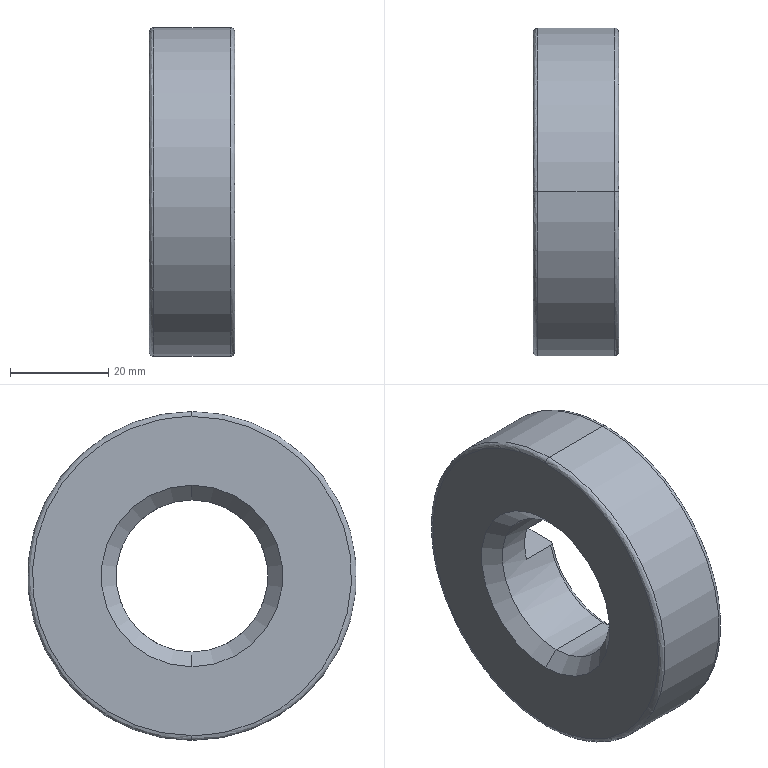Part | SolidWorks | features BaseBody 1 | 1 solid | 23 faces | box 17.5 x 67 x 67 mm | volume 46586 mm3 | plane 8 | spline 7 | cylinder 6 | cone 2 | commonest cylinder face diameters 7.5 x2 31 x2 67 x2
STEP:
#1=CARTESIAN_POINT('',(0.,0.,32.5));
#2=VERTEX_POINT('',#1);
#3=CARTESIAN_POINT('',(0.,0.,-32.5));
#4=VERTEX_POINT('',#3);
#5=CARTESIAN_POINT('',(0.,0.,32.5));
#6=CARTESIAN_POINT('',(0.,-65.,32.5));
#7=CARTESIAN_POINT('',(0.,-65.,-32.5));
#8=CARTESIAN_POINT('',(0.,0.,-32.5));
#9=(BOUNDED_CURVE()B_SPLINE_CURVE(3,(#5,#6,#7,#8),.UNSPECIFIED.,.F.,.T.)B_SPLINE_CURVE_WITH_KNOTS((4,4),(0.25,0.75),.UNSPECIFIED.)CURVE()GEOMETRIC_REPRESENTATION_ITEM()RATIONAL_B_SPLINE_CURVE((1.,0.3333,0.3333,1.))REPRESENTATION_ITEM(''));
#10=EDGE_CURVE('',#2,#4,#9,.T.);
#11=ORIENTED_EDGE('',*,*,#10,.T.);
#12=CARTESIAN_POINT('',(1.,0.,-33.5));
#13=VERTEX_POINT('',#12);
#14=CARTESIAN_POINT('',(1.,0.,-32.5));
#15=DIRECTION('',(0.,-1.,0.));
#16=DIRECTION('',(0.,0.,-1.));
#17=AXIS2_PLACEMENT_3D('',#14,#15,#16);
#18=CIRCLE('',#17,1.);
#19=EDGE_CURVE('',#4,#13,#18,.T.);
#20=ORIENTED_EDGE('',*,*,#19,.T.);
#21=CARTESIAN_POINT('',(1.,0.,33.5));
#22=VERTEX_POINT('',#21);
#23=CARTESIAN_POINT('',(1.,0.,0.));
#24=DIRECTION('',(1.,0.,0.));
#25=DIRECTION('',(0.,0.,-1.));
#26=AXIS2_PLACEMENT_3D('',#23,#24,#25);
#27=CIRCLE('',#26,33.5);
#28=EDGE_CURVE('',#22,#13,#27,.T.);
#29=ORIENTED_EDGE('',*,*,#28,.F.);
#30=CARTESIAN_POINT('',(1.,0.,32.5));
#31=DIRECTION('',(0.,1.,0.));
#32=DIRECTION('',(0.,0.,1.));
#33=AXIS2_PLACEMENT_3D('',#30,#31,#32);
#34=CIRCLE('',#33,1.);
#35=EDGE_CURVE('',#2,#22,#34,.T.);
#36=ORIENTED_EDGE('',*,*,#35,.F.);
#37=EDGE_LOOP('',(#11,#20,#29,#36));
#38=FACE_OUTER_BOUND('',#37,.T.);
#39=CARTESIAN_POINT('',(0.,0.,-32.5));
#40=CARTESIAN_POINT('',(0.,-65.,-32.5));
#41=CARTESIAN_POINT('',(0.,-65.,32.5));
#42=CARTESIAN_POINT('',(0.,0.,32.5));
#43=CARTESIAN_POINT('',(0.,0.,-33.086));
#44=CARTESIAN_POINT('',(0.,-66.172,-33.086));
#45=CARTESIAN_POINT('',(0.,-66.172,33.086));
#46=CARTESIAN_POINT('',(0.,0.,33.086));
#47=CARTESIAN_POINT('',(0.4142,0.,-33.5));
#48=CARTESIAN_POINT('',(0.4142,-67.,-33.5));
#49=CARTESIAN_POINT('',(0.4142,-67.,33.5));
#50=CARTESIAN_POINT('',(0.4142,0.,33.5));
#51=CARTESIAN_POINT('',(1.,0.,-33.5));
#52=CARTESIAN_POINT('',(1.,-67.,-33.5));
#53=CARTESIAN_POINT('',(1.,-67.,33.5));
#54=CARTESIAN_POINT('',(1.,0.,33.5));
#55=(BOUNDED_SURFACE()B_SPLINE_SURFACE(3,3,((#39,#40,#41,#42),(#43,#44,#45,#46),(#47,#48,#49,#50),(#51,#52,#53,#54)),.UNSPECIFIED.,.F.,.F.,.T.)B_SPLINE_SURFACE_WITH_KNOTS((4,4),(4,4),(0.,1.),(0.,1.),.UNSPECIFIED.)GEOMETRIC_REPRESENTATION_ITEM()RATIONAL_B_SPLINE_SURFACE(((1.,0.3333,0.3333,1.),(0.8047,0.2682,0.2682,0.8047),(0.8047,0.2682,0.2682,0.8047),(1.,0.3333,0.3333,1.)))REPRESENTATION_ITEM('')SURFACE());
#56=ADVANCED_FACE('',(#38),#55,.T.);
#57=CARTESIAN_POINT('',(17.5,0.,-32.5));
#58=VERTEX_POINT('',#57);
#59=CARTESIAN_POINT('',(17.5,0.,32.5));
#60=VERTEX_POINT('',#59);
#61=CARTESIAN_POINT('',(17.5,0.,-32.5));
#62=CARTESIAN_POINT('',(17.5,-65.,-32.5));
#63=CARTESIAN_POINT('',(17.5,-65.,32.5));
#64=CARTESIAN_POINT('',(17.5,0.,32.5));
#65=(BOUNDED_CURVE()B_SPLINE_CURVE(3,(#61,#62,#63,#64),.UNSPECIFIED.,.F.,.T.)B_SPLINE_CURVE_WITH_KNOTS((4,4),(0.25,0.75),.UNSPECIFIED.)CURVE()GEOMETRIC_REPRESENTATION_ITEM()RATIONAL_B_SPLINE_CURVE((1.,0.3333,0.3333,1.))REPRESENTATION_ITEM(''));
#66=EDGE_CURVE('',#58,#60,#65,.T.);
#67=ORIENTED_EDGE('',*,*,#66,.T.);
#68=CARTESIAN_POINT('',(16.5,0.,33.5));
#69=VERTEX_POINT('',#68);
#70=CARTESIAN_POINT('',(16.5,0.,32.5));
#71=DIRECTION('',(0.,-1.,0.));
#72=DIRECTION('',(0.,0.,1.));
#73=AXIS2_PLACEMENT_3D('',#70,#71,#72);
#74=CIRCLE('',#73,1.);
#75=EDGE_CURVE('',#60,#69,#74,.T.);
#76=ORIENTED_EDGE('',*,*,#75,.T.);
#77=CARTESIAN_POINT('',(16.5,0.,-33.5));
#78=VERTEX_POINT('',#77);
#79=CARTESIAN_POINT('',(16.5,0.,0.));
#80=DIRECTION('',(-1.,0.,0.));
#81=DIRECTION('',(0.,0.,-1.));
#82=AXIS2_PLACEMENT_3D('',#79,#80,#81);
#83=CIRCLE('',#82,33.5);
#84=EDGE_CURVE('',#78,#69,#83,.T.);
#85=ORIENTED_EDGE('',*,*,#84,.F.);
#86=CARTESIAN_POINT('',(16.5,0.,-32.5));
#87=DIRECTION('',(0.,1.,0.));
#88=DIRECTION('',(0.,0.,-1.));
#89=AXIS2_PLACEMENT_3D('',#86,#87,#88);
#90=CIRCLE('',#89,1.);
#91=EDGE_CURVE('',#58,#78,#90,.T.);
#92=ORIENTED_EDGE('',*,*,#91,.F.);
#93=EDGE_LOOP('',(#67,#76,#85,#92));
#94=FACE_OUTER_BOUND('',#93,.T.);
#95=CARTESIAN_POINT('',(17.5,0.,32.5));
#96=CARTESIAN_POINT('',(17.5,-65.,32.5));
#97=CARTESIAN_POINT('',(17.5,-65.,-32.5));
#98=CARTESIAN_POINT('',(17.5,0.,-32.5));
#99=CARTESIAN_POINT('',(17.5,0.,33.086));
#100=CARTESIAN_POINT('',(17.5,-66.172,33.086));
#101=CARTESIAN_POINT('',(17.5,-66.172,-33.086));
#102=CARTESIAN_POINT('',(17.5,0.,-33.086));
#103=CARTESIAN_POINT('',(17.086,0.,33.5));
#104=CARTESIAN_POINT('',(17.086,-67.,33.5));
#105=CARTESIAN_POINT('',(17.086,-67.,-33.5));
#106=CARTESIAN_POINT('',(17.086,0.,-33.5));
#107=CARTESIAN_POINT('',(16.5,0.,33.5));
#108=CARTESIAN_POINT('',(16.5,-67.,33.5));
#109=CARTESIAN_POINT('',(16.5,-67.,-33.5));
#110=CARTESIAN_POINT('',(16.5,0.,-33.5));
#111=(BOUNDED_SURFACE()B_SPLINE_SURFACE(3,3,((#95,#96,#97,#98),(#99,#100,#101,#102),(#103,#104,#105,#106),(#107,#108,#109,#110)),.UNSPECIFIED.,.F.,.F.,.F.)B_SPLINE_SURFACE_WITH_KNOTS((4,4),(4,4),(0.,1.),(0.,1.),.UNSPECIFIED.)GEOMETRIC_REPRESENTATION_ITEM()RATIONAL_B_SPLINE_SURFACE(((1.,0.3333,0.3333,1.),(0.8047,0.2682,0.2682,0.8047),(0.8047,0.2682,0.2682,0.8047),(1.,0.3333,0.3333,1.)))REPRESENTATION_ITEM('')SURFACE());
#112=ADVANCED_FACE('',(#94),#111,.T.);
#113=CARTESIAN_POINT('',(17.5,0.,16.5));
#114=VERTEX_POINT('',#113);
#115=CARTESIAN_POINT('',(17.5,16.068,3.75));
#116=VERTEX_POINT('',#115);
#117=CARTESIAN_POINT('',(17.5,0.,16.5));
#118=CARTESIAN_POINT('',(17.5,0.4391,16.5));
#119=CARTESIAN_POINT('',(17.5,1.096,16.474));
#120=CARTESIAN_POINT('',(17.5,1.858,16.398));
#121=CARTESIAN_POINT('',(17.5,2.239,16.348));
#122=CARTESIAN_POINT('',(17.5,2.429,16.32));
#123=CARTESIAN_POINT('',(17.5,2.51,16.308));
#124=CARTESIAN_POINT('',(17.5,2.564,16.3));
#125=CARTESIAN_POINT('',(17.5,2.59,16.295));
#126=CARTESIAN_POINT('',(17.5,3.071,16.218));
#127=CARTESIAN_POINT('',(17.5,3.743,16.081));
#128=CARTESIAN_POINT('',(17.5,4.515,15.873));
#129=CARTESIAN_POINT('',(17.5,4.898,15.757));
#130=CARTESIAN_POINT('',(17.5,5.062,15.705));
#131=CARTESIAN_POINT('',(17.5,5.171,15.669));
#132=CARTESIAN_POINT('',(17.5,5.223,15.652));
#133=CARTESIAN_POINT('',(17.5,5.726,15.482));
#134=CARTESIAN_POINT('',(17.5,6.385,15.227));
#135=CARTESIAN_POINT('',(17.5,7.132,14.882));
#136=CARTESIAN_POINT('',(17.5,7.448,14.724));
#137=CARTESIAN_POINT('',(17.5,7.658,14.616));
#138=CARTESIAN_POINT('',(17.5,7.761,14.561));
#139=CARTESIAN_POINT('',(17.5,8.708,14.048));
#140=CARTESIAN_POINT('',(17.5,9.506,13.521));
#141=CARTESIAN_POINT('',(17.5,10.631,12.627));
#142=CARTESIAN_POINT('',(17.5,11.173,12.158));
#143=CARTESIAN_POINT('',(17.5,11.767,11.571));
#144=CARTESIAN_POINT('',(17.5,12.014,11.31));
#145=CARTESIAN_POINT('',(17.5,12.177,11.135));
#146=CARTESIAN_POINT('',(17.5,12.259,11.045));
#147=CARTESIAN_POINT('',(17.5,12.65,10.604));
#148=CARTESIAN_POINT('',(17.5,13.096,10.056));
#149=CARTESIAN_POINT('',(17.5,13.574,9.386));
#150=CARTESIAN_POINT('',(17.5,13.802,9.042));
#151=CARTESIAN_POINT('',(17.5,13.898,8.894));
#152=CARTESIAN_POINT('',(17.5,13.961,8.794));
#153=CARTESIAN_POINT('',(17.5,13.994,8.743));
#154=CARTESIAN_POINT('',(17.5,14.265,8.305));
#155=CARTESIAN_POINT('',(17.5,14.602,7.707));
#156=CARTESIAN_POINT('',(17.5,14.95,6.988));
#157=CARTESIAN_POINT('',(17.5,15.114,6.622));
#158=CARTESIAN_POINT('',(17.5,15.192,6.438));
#159=CARTESIAN_POINT('',(17.5,15.226,6.359));
#160=CARTESIAN_POINT('',(17.5,15.248,6.306));
#161=CARTESIAN_POINT('',(17.5,15.259,6.278));
#162=CARTESIAN_POINT('',(17.5,15.602,5.44));
#163=CARTESIAN_POINT('',(17.5,15.868,4.606));
#164=CARTESIAN_POINT('',(17.5,16.068,3.75));
#165=B_SPLINE_CURVE_WITH_KNOTS('',3,(#117,#118,#119,#120,#121,#122,#123,#124,#125,#126,#127,#128,#129,#130,#131,#132,#133,#134,#135,#136,#137,#138,#139,#140,#141,#142,#143,#144,#145,#146,#147,#148,#149,#150,#151,#152,#153,#154,#155,#156,#157,#158,#159,#160,#161,#162,#163,#164),.UNSPECIFIED.,.F.,.F.,(4,1,1,1,1,2,2,1,1,1,2,2,1,1,2,2,2,1,1,2,2,1,1,1,2,2,1,1,1,1,2,2,4),(0.5,0.5312,0.5469,0.5547,0.5586,0.5605,0.5625,0.5938,0.6094,0.6172,0.6211,0.625,0.6562,0.6719,0.6797,0.6875,0.75,0.7812,0.7969,0.8047,0.8125,0.8437,0.8594,0.8672,0.8711,0.875,0.9062,0.9219,0.9297,0.9336,0.9355,0.9375,1.),.UNSPECIFIED.);
#166=EDGE_CURVE('',#114,#116,#165,.T.);
#167=ORIENTED_EDGE('',*,*,#166,.F.);
#168=CARTESIAN_POINT('',(16.5,0.,15.5));
#169=VERTEX_POINT('',#168);
#170=CARTESIAN_POINT('',(16.5,0.,16.5));
#171=DIRECTION('',(0.,1.,0.));
#172=DIRECTION('',(0.,0.,1.));
#173=AXIS2_PLACEMENT_3D('',#170,#171,#172);
#174=CIRCLE('',#173,1.);
#175=EDGE_CURVE('',#114,#169,#174,.T.);
#176=ORIENTED_EDGE('',*,*,#175,.T.);
#177=CARTESIAN_POINT('',(16.5,15.04,3.75));
#178=VERTEX_POINT('',#177);
#179=CARTESIAN_POINT('',(16.5,0.,0.));
#180=DIRECTION('',(-1.,0.,0.));
#181=DIRECTION('',(0.,0.,1.));
#182=AXIS2_PLACEMENT_3D('',#179,#180,#181);
#183=CIRCLE('',#182,15.5);
#184=EDGE_CURVE('',#169,#178,#183,.T.);
#185=ORIENTED_EDGE('',*,*,#184,.T.);
#186=CARTESIAN_POINT('',(16.5,15.04,3.75));
#187=CARTESIAN_POINT('',(16.634,15.04,3.75));
#188=CARTESIAN_POINT('',(16.765,15.067,3.75));
#189=CARTESIAN_POINT('',(17.009,15.173,3.75));
#190=CARTESIAN_POINT('',(17.12,15.251,3.75));
#191=CARTESIAN_POINT('',(17.303,15.441,3.75));
#192=CARTESIAN_POINT('',(17.376,15.556,3.75));
#193=CARTESIAN_POINT('',(17.474,15.801,3.75));
#194=CARTESIAN_POINT('',(17.5,15.934,3.75));
#195=CARTESIAN_POINT('',(17.5,16.068,3.75));
#196=B_SPLINE_CURVE_WITH_KNOTS('',3,(#186,#187,#188,#189,#190,#191,#192,#193,#194,#195),.UNSPECIFIED.,.F.,.F.,(4,2,2,2,4),(0.,0.0003961,0.0007922,0.001188,0.001584),.UNSPECIFIED.);
#197=EDGE_CURVE('',#178,#116,#196,.T.);
#198=ORIENTED_EDGE('',*,*,#197,.T.);
#199=EDGE_LOOP('',(#167,#176,#185,#198));
#200=FACE_OUTER_BOUND('',#199,.T.);
#201=CARTESIAN_POINT('',(17.5,0.,16.5));
#202=CARTESIAN_POINT('',(17.5,8.048,16.5));
#203=CARTESIAN_POINT('',(17.5,14.332,11.472));
#204=CARTESIAN_POINT('',(17.5,16.098,3.621));
#205=CARTESIAN_POINT('',(17.5,0.,15.914));
#206=CARTESIAN_POINT('',(17.5,7.762,15.914));
#207=CARTESIAN_POINT('',(17.5,13.823,11.065));
#208=CARTESIAN_POINT('',(17.5,15.526,3.492));
#209=CARTESIAN_POINT('',(17.086,0.,15.5));
#210=CARTESIAN_POINT('',(17.086,7.56,15.5));
#211=CARTESIAN_POINT('',(17.086,13.463,10.777));
#212=CARTESIAN_POINT('',(17.086,15.122,3.401));
#213=CARTESIAN_POINT('',(16.5,0.,15.5));
#214=CARTESIAN_POINT('',(16.5,7.56,15.5));
#215=CARTESIAN_POINT('',(16.5,13.463,10.777));
#216=CARTESIAN_POINT('',(16.5,15.122,3.401));
#217=(BOUNDED_SURFACE()B_SPLINE_SURFACE(3,3,((#201,#202,#203,#204),(#205,#206,#207,#208),(#209,#210,#211,#212),(#213,#214,#215,#216)),.UNSPECIFIED.,.F.,.F.,.T.)B_SPLINE_SURFACE_WITH_KNOTS((4,4),(4,4),(0.,1.),(0.,1.),.UNSPECIFIED.)GEOMETRIC_REPRESENTATION_ITEM()RATIONAL_B_SPLINE_SURFACE(((1.,0.8539,0.8539,1.),(0.8047,0.6872,0.6872,0.8047),(0.8047,0.6872,0.6872,0.8047),(1.,0.8539,0.8539,1.)))REPRESENTATION_ITEM('')SURFACE());
#218=ADVANCED_FACE('',(#200),#217,.T.);
#219=CARTESIAN_POINT('',(1.,0.,0.));
#220=DIRECTION('',(1.,0.,0.));
#221=DIRECTION('',(0.,0.,-1.));
#222=AXIS2_PLACEMENT_3D('',#219,#220,#221);
#223=CIRCLE('',#222,33.5);
#224=EDGE_CURVE('',#13,#22,#223,.T.);
#225=ORIENTED_EDGE('',*,*,#224,.T.);
#226=CARTESIAN_POINT('',(0.,0.,33.5));
#227=DIRECTION('',(1.,0.,0.));
#228=VECTOR('',#227,1000.);
#229=LINE('',#226,#228);
#230=EDGE_CURVE('',#22,#69,#229,.T.);
#231=ORIENTED_EDGE('',*,*,#230,.T.);
#232=CARTESIAN_POINT('',(16.5,0.,0.));
#233=DIRECTION('',(-1.,0.,0.));
#234=DIRECTION('',(0.,0.,-1.));
#235=AXIS2_PLACEMENT_3D('',#232,#233,#234);
#236=CIRCLE('',#235,33.5);
#237=EDGE_CURVE('',#69,#78,#236,.T.);
#238=ORIENTED_EDGE('',*,*,#237,.T.);
#239=CARTESIAN_POINT('',(0.,0.,-33.5));
#240=DIRECTION('',(1.,0.,0.));
#241=VECTOR('',#240,1000.);
#242=LINE('',#239,#241);
#243=EDGE_CURVE('',#13,#78,#242,.T.);
#244=ORIENTED_EDGE('',*,*,#243,.F.);
#245=EDGE_LOOP('',(#225,#231,#238,#244));
#246=FACE_OUTER_BOUND('',#245,.T.);
#247=CARTESIAN_POINT('',(0.,0.,0.));
#248=DIRECTION('',(1.,0.,0.));
#249=DIRECTION('',(0.,0.,-1.));
#250=AXIS2_PLACEMENT_3D('',#247,#248,#249);
#251=CYLINDRICAL_SURFACE('',#250,33.5);
#252=ADVANCED_FACE('',(#246),#251,.T.);
#253=CARTESIAN_POINT('',(3.,0.,-15.5));
#254=VERTEX_POINT('',#253);
#255=CARTESIAN_POINT('',(3.,0.,15.5));
#256=VERTEX_POINT('',#255);
#257=CARTESIAN_POINT('',(3.,0.,0.));
#258=DIRECTION('',(-1.,0.,0.));
#259=DIRECTION('',(0.,-1.,0.));
#260=AXIS2_PLACEMENT_3D('',#257,#258,#259);
#261=CIRCLE('',#260,15.5);
#262=EDGE_CURVE('',#254,#256,#261,.T.);
#263=ORIENTED_EDGE('',*,*,#262,.F.);
#264=CARTESIAN_POINT('',(0.,0.,-18.5));
#265=VERTEX_POINT('',#264);
#266=CARTESIAN_POINT('',(0.,0.,-18.5));
#267=DIRECTION('',(-0.7071,0.,-0.7071));
#268=VECTOR('',#267,1000.);
#269=LINE('',#266,#268);
#270=EDGE_CURVE('',#254,#265,#269,.T.);
#271=ORIENTED_EDGE('',*,*,#270,.T.);
#272=CARTESIAN_POINT('',(0.,0.,18.5));
#273=VERTEX_POINT('',#272);
#274=CARTESIAN_POINT('',(0.,0.,0.));
#275=DIRECTION('',(-1.,0.,0.));
#276=DIRECTION('',(0.,0.,1.));
#277=AXIS2_PLACEMENT_3D('',#274,#275,#276);
#278=CIRCLE('',#277,18.5);
#279=EDGE_CURVE('',#265,#273,#278,.T.);
#280=ORIENTED_EDGE('',*,*,#279,.T.);
#281=CARTESIAN_POINT('',(0.,0.,18.5));
#282=DIRECTION('',(-0.7071,0.,0.7071));
#283=VECTOR('',#282,1000.);
#284=LINE('',#281,#283);
#285=EDGE_CURVE('',#256,#273,#284,.T.);
#286=ORIENTED_EDGE('',*,*,#285,.F.);
#287=EDGE_LOOP('',(#263,#271,#280,#286));
#288=FACE_OUTER_BOUND('',#287,.T.);
#289=CARTESIAN_POINT('',(0.,0.,0.));
#290=DIRECTION('',(-1.,0.,0.));
#291=DIRECTION('',(0.,0.,1.));
#292=AXIS2_PLACEMENT_3D('',#289,#290,#291);
#293=CONICAL_SURFACE('',#292,18.5,0.7854);
#294=ADVANCED_FACE('',(#288),#293,.F.);
#295=ORIENTED_EDGE('',*,*,#262,.T.);
#296=CARTESIAN_POINT('',(0.,0.,15.5));
#297=DIRECTION('',(1.,0.,0.));
#298=VECTOR('',#297,1000.);
#299=LINE('',#296,#298);
#300=EDGE_CURVE('',#256,#169,#299,.T.);
#301=ORIENTED_EDGE('',*,*,#300,.T.);
#302=CARTESIAN_POINT('',(16.5,-15.04,3.75));
#303=VERTEX_POINT('',#302);
#304=CARTESIAN_POINT('',(16.5,0.,0.));
#305=DIRECTION('',(-1.,0.,0.));
#306=DIRECTION('',(0.,0.,1.));
#307=AXIS2_PLACEMENT_3D('',#304,#305,#306);
#308=CIRCLE('',#307,15.5);
#309=EDGE_CURVE('',#303,#169,#308,.T.);
#310=ORIENTED_EDGE('',*,*,#309,.F.);
#311=CARTESIAN_POINT('',(9.5,-15.04,3.75));
#312=VERTEX_POINT('',#311);
#313=CARTESIAN_POINT('',(17.5,-15.04,3.75));
#314=DIRECTION('',(-1.,0.,0.));
#315=VECTOR('',#314,1000.);
#316=LINE('',#313,#315);
#317=EDGE_CURVE('',#303,#312,#316,.T.);
#318=ORIENTED_EDGE('',*,*,#317,.T.);
#319=CARTESIAN_POINT('',(9.5,-15.04,-3.75));
#320=VERTEX_POINT('',#319);
#321=CARTESIAN_POINT('',(9.5,0.,0.));
#322=DIRECTION('',(-1.,0.,0.));
#323=DIRECTION('',(0.,0.,-1.));
#324=AXIS2_PLACEMENT_3D('',#321,#322,#323);
#325=CIRCLE('',#324,15.5);
#326=EDGE_CURVE('',#320,#312,#325,.T.);
#327=ORIENTED_EDGE('',*,*,#326,.F.);
#328=CARTESIAN_POINT('',(16.5,-15.04,-3.75));
#329=VERTEX_POINT('',#328);
#330=CARTESIAN_POINT('',(17.5,-15.04,-3.75));
#331=DIRECTION('',(1.,0.,0.));
#332=VECTOR('',#331,1000.);
#333=LINE('',#330,#332);
#334=EDGE_CURVE('',#320,#329,#333,.T.);
#335=ORIENTED_EDGE('',*,*,#334,.T.);
#336=CARTESIAN_POINT('',(16.5,0.,-15.5));
#337=VERTEX_POINT('',#336);
#338=CARTESIAN_POINT('',(16.5,0.,0.));
#339=DIRECTION('',(-1.,0.,0.));
#340=DIRECTION('',(0.,0.,1.));
#341=AXIS2_PLACEMENT_3D('',#338,#339,#340);
#342=CIRCLE('',#341,15.5);
#343=EDGE_CURVE('',#337,#329,#342,.T.);
#344=ORIENTED_EDGE('',*,*,#343,.F.);
#345=CARTESIAN_POINT('',(0.,0.,-15.5));
#346=DIRECTION('',(1.,0.,0.));
#347=VECTOR('',#346,1000.);
#348=LINE('',#345,#347);
#349=EDGE_CURVE('',#254,#337,#348,.T.);
#350=ORIENTED_EDGE('',*,*,#349,.F.);
#351=EDGE_LOOP('',(#295,#301,#310,#318,#327,#335,#344,#350));
#352=FACE_OUTER_BOUND('',#351,.T.);
#353=CARTESIAN_POINT('',(0.,0.,0.));
#354=DIRECTION('',(1.,0.,0.));
#355=DIRECTION('',(0.,0.,-1.));
#356=AXIS2_PLACEMENT_3D('',#353,#354,#355);
#357=CYLINDRICAL_SURFACE('',#356,15.5);
#358=ADVANCED_FACE('',(#352),#357,.F.);
#359=ORIENTED_EDGE('',*,*,#230,.F.);
#360=ORIENTED_EDGE('',*,*,#28,.T.);
#361=ORIENTED_EDGE('',*,*,#243,.T.);
#362=ORIENTED_EDGE('',*,*,#84,.T.);
#363=EDGE_LOOP('',(#359,#360,#361,#362));
#364=FACE_OUTER_BOUND('',#363,.T.);
#365=CARTESIAN_POINT('',(0.,0.,0.));
#366=DIRECTION('',(1.,0.,0.));
#367=DIRECTION('',(0.,0.,-1.));
#368=AXIS2_PLACEMENT_3D('',#365,#366,#367);
#369=CYLINDRICAL_SURFACE('',#368,33.5);
#370=ADVANCED_FACE('',(#364),#369,.T.);
#371=ORIENTED_EDGE('',*,*,#19,.F.);
#372=CARTESIAN_POINT('',(0.,0.,-32.5));
#373=CARTESIAN_POINT('',(0.,65.,-32.5));
#374=CARTESIAN_POINT('',(0.,65.,32.5));
#375=CARTESIAN_POINT('',(0.,0.,32.5));
#376=(BOUNDED_CURVE()B_SPLINE_CURVE(3,(#372,#373,#374,#375),.UNSPECIFIED.,.F.,.T.)B_SPLINE_CURVE_WITH_KNOTS((4,4),(0.75,1.25),.UNSPECIFIED.)CURVE()GEOMETRIC_REPRESENTATION_ITEM()RATIONAL_B_SPLINE_CURVE((1.,0.3333,0.3333,1.))REPRESENTATION_ITEM(''));
#377=EDGE_CURVE('',#4,#2,#376,.T.);
#378=ORIENTED_EDGE('',*,*,#377,.T.);
#379=ORIENTED_EDGE('',*,*,#35,.T.);
#380=ORIENTED_EDGE('',*,*,#224,.F.);
#381=EDGE_LOOP('',(#371,#378,#379,#380));
#382=FACE_OUTER_BOUND('',#381,.T.);
#383=CARTESIAN_POINT('',(0.,0.,32.5));
#384=CARTESIAN_POINT('',(0.,65.,32.5));
#385=CARTESIAN_POINT('',(0.,65.,-32.5));
#386=CARTESIAN_POINT('',(0.,0.,-32.5));
#387=CARTESIAN_POINT('',(0.,0.,33.086));
#388=CARTESIAN_POINT('',(0.,66.172,33.086));
#389=CARTESIAN_POINT('',(0.,66.172,-33.086));
#390=CARTESIAN_POINT('',(0.,0.,-33.086));
#391=CARTESIAN_POINT('',(0.4142,0.,33.5));
#392=CARTESIAN_POINT('',(0.4142,67.,33.5));
#393=CARTESIAN_POINT('',(0.4142,67.,-33.5));
#394=CARTESIAN_POINT('',(0.4142,0.,-33.5));
#395=CARTESIAN_POINT('',(1.,0.,33.5));
#396=CARTESIAN_POINT('',(1.,67.,33.5));
#397=CARTESIAN_POINT('',(1.,67.,-33.5));
#398=CARTESIAN_POINT('',(1.,0.,-33.5));
#399=(BOUNDED_SURFACE()B_SPLINE_SURFACE(3,3,((#383,#384,#385,#386),(#387,#388,#389,#390),(#391,#392,#393,#394),(#395,#396,#397,#398)),.UNSPECIFIED.,.F.,.F.,.T.)B_SPLINE_SURFACE_WITH_KNOTS((4,4),(4,4),(0.,1.),(0.,1.),.UNSPECIFIED.)GEOMETRIC_REPRESENTATION_ITEM()RATIONAL_B_SPLINE_SURFACE(((1.,0.3333,0.3333,1.),(0.8047,0.2682,0.2682,0.8047),(0.8047,0.2682,0.2682,0.8047),(1.,0.3333,0.3333,1.)))REPRESENTATION_ITEM('')SURFACE());
#400=ADVANCED_FACE('',(#382),#399,.T.);
#401=ORIENTED_EDGE('',*,*,#75,.F.);
#402=CARTESIAN_POINT('',(17.5,0.,32.5));
#403=CARTESIAN_POINT('',(17.5,65.,32.5));
#404=CARTESIAN_POINT('',(17.5,65.,-32.5));
#405=CARTESIAN_POINT('',(17.5,0.,-32.5));
#406=(BOUNDED_CURVE()B_SPLINE_CURVE(3,(#402,#403,#404,#405),.UNSPECIFIED.,.F.,.T.)B_SPLINE_CURVE_WITH_KNOTS((4,4),(0.75,1.25),.UNSPECIFIED.)CURVE()GEOMETRIC_REPRESENTATION_ITEM()RATIONAL_B_SPLINE_CURVE((1.,0.3333,0.3333,1.))REPRESENTATION_ITEM(''));
#407=EDGE_CURVE('',#60,#58,#406,.T.);
#408=ORIENTED_EDGE('',*,*,#407,.T.);
#409=ORIENTED_EDGE('',*,*,#91,.T.);
#410=ORIENTED_EDGE('',*,*,#237,.F.);
#411=EDGE_LOOP('',(#401,#408,#409,#410));
#412=FACE_OUTER_BOUND('',#411,.T.);
#413=CARTESIAN_POINT('',(17.5,0.,-32.5));
#414=CARTESIAN_POINT('',(17.5,65.,-32.5));
#415=CARTESIAN_POINT('',(17.5,65.,32.5));
#416=CARTESIAN_POINT('',(17.5,0.,32.5));
#417=CARTESIAN_POINT('',(17.5,0.,-33.086));
#418=CARTESIAN_POINT('',(17.5,66.172,-33.086));
#419=CARTESIAN_POINT('',(17.5,66.172,33.086));
#420=CARTESIAN_POINT('',(17.5,0.,33.086));
#421=CARTESIAN_POINT('',(17.086,0.,-33.5));
#422=CARTESIAN_POINT('',(17.086,67.,-33.5));
#423=CARTESIAN_POINT('',(17.086,67.,33.5));
#424=CARTESIAN_POINT('',(17.086,0.,33.5));
#425=CARTESIAN_POINT('',(16.5,0.,-33.5));
#426=CARTESIAN_POINT('',(16.5,67.,-33.5));
#427=CARTESIAN_POINT('',(16.5,67.,33.5));
#428=CARTESIAN_POINT('',(16.5,0.,33.5));
#429=(BOUNDED_SURFACE()B_SPLINE_SURFACE(3,3,((#413,#414,#415,#416),(#417,#418,#419,#420),(#421,#422,#423,#424),(#425,#426,#427,#428)),.UNSPECIFIED.,.F.,.F.,.T.)B_SPLINE_SURFACE_WITH_KNOTS((4,4),(4,4),(0.,1.),(0.,1.),.UNSPECIFIED.)GEOMETRIC_REPRESENTATION_ITEM()RATIONAL_B_SPLINE_SURFACE(((1.,0.3333,0.3333,1.),(0.8047,0.2682,0.2682,0.8047),(0.8047,0.2682,0.2682,0.8047),(1.,0.3333,0.3333,1.)))REPRESENTATION_ITEM('')SURFACE());
#430=ADVANCED_FACE('',(#412),#429,.T.);
#431=CARTESIAN_POINT('',(0.,0.,0.));
#432=DIRECTION('',(-1.,0.,0.));
#433=DIRECTION('',(0.,0.,1.));
#434=AXIS2_PLACEMENT_3D('',#431,#432,#433);
#435=CIRCLE('',#434,18.5);
#436=EDGE_CURVE('',#273,#265,#435,.T.);
#437=ORIENTED_EDGE('',*,*,#436,.F.);
#438=ORIENTED_EDGE('',*,*,#279,.F.);
#439=EDGE_LOOP('',(#437,#438));
#440=FACE_BOUND('',#439,.T.);
#441=ORIENTED_EDGE('',*,*,#10,.F.);
#442=ORIENTED_EDGE('',*,*,#377,.F.);
#443=EDGE_LOOP('',(#441,#442));
#444=FACE_OUTER_BOUND('',#443,.T.);
#445=CARTESIAN_POINT('',(0.,0.,0.));
#446=DIRECTION('',(1.,0.,0.));
#447=DIRECTION('',(0.,0.,-1.));
#448=AXIS2_PLACEMENT_3D('',#445,#446,#447);
#449=PLANE('',#448);
#450=ADVANCED_FACE('',(#440,#444),#449,.F.);
#451=CARTESIAN_POINT('',(17.5,-23.5,-3.75));
#452=VERTEX_POINT('',#451);
#453=CARTESIAN_POINT('',(17.5,-23.5,3.75));
#454=VERTEX_POINT('',#453);
#455=CARTESIAN_POINT('',(17.5,-23.5,0.));
#456=DIRECTION('',(-1.,0.,0.));
#457=DIRECTION('',(0.,0.,1.));
#458=AXIS2_PLACEMENT_3D('',#455,#456,#457);
#459=CIRCLE('',#458,3.75);
#460=EDGE_CURVE('',#452,#454,#459,.T.);
#461=ORIENTED_EDGE('',*,*,#460,.T.);
#462=CARTESIAN_POINT('',(17.5,-16.068,3.75));
#463=VERTEX_POINT('',#462);
#464=CARTESIAN_POINT('',(17.5,0.,3.75));
#465=DIRECTION('',(0.,1.,0.));
#466=VECTOR('',#465,1000.);
#467=LINE('',#464,#466);
#468=EDGE_CURVE('',#454,#463,#467,.T.);
#469=ORIENTED_EDGE('',*,*,#468,.T.);
#470=CARTESIAN_POINT('',(17.5,-16.068,3.75));
#471=CARTESIAN_POINT('',(17.5,-15.968,4.178));
#472=CARTESIAN_POINT('',(17.5,-15.794,4.811));
#473=CARTESIAN_POINT('',(17.5,-15.546,5.537));
#474=CARTESIAN_POINT('',(17.5,-15.411,5.896));
#475=CARTESIAN_POINT('',(17.5,-15.341,6.075));
#476=CARTESIAN_POINT('',(17.5,-15.311,6.151));
#477=CARTESIAN_POINT('',(17.5,-15.29,6.202));
#478=CARTESIAN_POINT('',(17.5,-15.28,6.226));
#479=CARTESIAN_POINT('',(17.5,-15.096,6.677));
#480=CARTESIAN_POINT('',(17.5,-14.81,7.3));
#481=CARTESIAN_POINT('',(17.5,-14.432,8.004));
#482=CARTESIAN_POINT('',(17.5,-14.231,8.351));
#483=CARTESIAN_POINT('',(17.5,-14.143,8.498));
#484=CARTESIAN_POINT('',(17.5,-14.084,8.596));
#485=CARTESIAN_POINT('',(17.5,-14.055,8.644));
#486=CARTESIAN_POINT('',(17.5,-13.775,9.095));
#487=CARTESIAN_POINT('',(17.5,-13.378,9.679));
#488=CARTESIAN_POINT('',(17.5,-12.872,10.328));
#489=CARTESIAN_POINT('',(17.5,-12.646,10.6));
#490=CARTESIAN_POINT('',(17.5,-12.493,10.779));
#491=CARTESIAN_POINT('',(17.5,-12.417,10.867));
#492=CARTESIAN_POINT('',(17.5,-11.701,11.673));
#493=CARTESIAN_POINT('',(17.5,-11.007,12.33));
#494=CARTESIAN_POINT('',(17.5,-9.881,13.223));
#495=CARTESIAN_POINT('',(17.5,-9.301,13.644));
#496=CARTESIAN_POINT('',(17.5,-8.593,14.089));
#497=CARTESIAN_POINT('',(17.5,-8.284,14.27));
#498=CARTESIAN_POINT('',(17.5,-8.076,14.389));
#499=CARTESIAN_POINT('',(17.5,-7.97,14.448));
#500=CARTESIAN_POINT('',(17.5,-7.451,14.729));
#501=CARTESIAN_POINT('',(17.5,-6.817,15.039));
#502=CARTESIAN_POINT('',(17.5,-6.055,15.352));
#503=CARTESIAN_POINT('',(17.5,-5.669,15.496));
#504=CARTESIAN_POINT('',(17.5,-5.502,15.556));
#505=CARTESIAN_POINT('',(17.5,-5.391,15.595));
#506=CARTESIAN_POINT('',(17.5,-5.333,15.614));
#507=CARTESIAN_POINT('',(17.5,-4.845,15.779));
#508=CARTESIAN_POINT('',(17.5,-4.187,15.972));
#509=CARTESIAN_POINT('',(17.5,-3.407,16.147));
#510=CARTESIAN_POINT('',(17.5,-3.014,16.223));
#511=CARTESIAN_POINT('',(17.5,-2.817,16.258));
#512=CARTESIAN_POINT('',(17.5,-2.732,16.272));
#513=CARTESIAN_POINT('',(17.5,-2.675,16.282));
#514=CARTESIAN_POINT('',(17.5,-2.646,16.287));
#515=CARTESIAN_POINT('',(17.5,-1.752,16.43));
#516=CARTESIAN_POINT('',(17.5,-0.8781,16.5));
#517=CARTESIAN_POINT('',(17.5,0.,16.5));
#518=B_SPLINE_CURVE_WITH_KNOTS('',3,(#470,#471,#472,#473,#474,#475,#476,#477,#478,#479,#480,#481,#482,#483,#484,#485,#486,#487,#488,#489,#490,#491,#492,#493,#494,#495,#496,#497,#498,#499,#500,#501,#502,#503,#504,#505,#506,#507,#508,#509,#510,#511,#512,#513,#514,#515,#516,#517),.UNSPECIFIED.,.F.,.F.,(4,1,1,1,1,2,2,1,1,1,2,2,1,1,2,2,2,1,1,2,2,1,1,1,2,2,1,1,1,1,2,2,4),(0.,0.03125,0.04688,0.05469,0.05859,0.06055,0.0625,0.09375,0.1094,0.1172,0.1211,0.125,0.1563,0.1719,0.1797,0.1875,0.25,0.2813,0.2969,0.3047,0.3125,0.3438,0.3594,0.3672,0.3711,0.375,0.4063,0.4219,0.4297,0.4336,0.4355,0.4375,0.5),.UNSPECIFIED.);
#519=EDGE_CURVE('',#463,#114,#518,.T.);
#520=ORIENTED_EDGE('',*,*,#519,.T.);
#521=ORIENTED_EDGE('',*,*,#166,.T.);
#522=CARTESIAN_POINT('',(17.5,23.5,3.75));
#523=VERTEX_POINT('',#522);
#524=CARTESIAN_POINT('',(17.5,0.,3.75));
#525=DIRECTION('',(0.,1.,0.));
#526=VECTOR('',#525,1000.);
#527=LINE('',#524,#526);
#528=EDGE_CURVE('',#116,#523,#527,.T.);
#529=ORIENTED_EDGE('',*,*,#528,.T.);
#530=CARTESIAN_POINT('',(17.5,23.5,-3.75));
#531=VERTEX_POINT('',#530);
#532=CARTESIAN_POINT('',(17.5,23.5,0.));
#533=DIRECTION('',(-1.,0.,0.));
#534=DIRECTION('',(0.,0.,1.));
#535=AXIS2_PLACEMENT_3D('',#532,#533,#534);
#536=CIRCLE('',#535,3.75);
#537=EDGE_CURVE('',#523,#531,#536,.T.);
#538=ORIENTED_EDGE('',*,*,#537,.T.);
#539=CARTESIAN_POINT('',(17.5,16.068,-3.75));
#540=VERTEX_POINT('',#539);
#541=CARTESIAN_POINT('',(17.5,0.,-3.75));
#542=DIRECTION('',(0.,-1.,0.));
#543=VECTOR('',#542,1000.);
#544=LINE('',#541,#543);
#545=EDGE_CURVE('',#531,#540,#544,.T.);
#546=ORIENTED_EDGE('',*,*,#545,.T.);
#547=CARTESIAN_POINT('',(17.5,-16.068,-3.75));
#548=VERTEX_POINT('',#547);
#549=CARTESIAN_POINT('',(17.5,16.068,-3.75));
#550=CARTESIAN_POINT('',(17.5,15.968,-4.178));
#551=CARTESIAN_POINT('',(17.5,15.794,-4.811));
#552=CARTESIAN_POINT('',(17.5,15.546,-5.537));
#553=CARTESIAN_POINT('',(17.5,15.411,-5.896));
#554=CARTESIAN_POINT('',(17.5,15.341,-6.075));
#555=CARTESIAN_POINT('',(17.5,15.311,-6.151));
#556=CARTESIAN_POINT('',(17.5,15.29,-6.202));
#557=CARTESIAN_POINT('',(17.5,15.28,-6.226));
#558=CARTESIAN_POINT('',(17.5,15.096,-6.677));
#559=CARTESIAN_POINT('',(17.5,14.81,-7.3));
#560=CARTESIAN_POINT('',(17.5,14.432,-8.004));
#561=CARTESIAN_POINT('',(17.5,14.231,-8.351));
#562=CARTESIAN_POINT('',(17.5,14.143,-8.498));
#563=CARTESIAN_POINT('',(17.5,14.084,-8.596));
#564=CARTESIAN_POINT('',(17.5,14.055,-8.644));
#565=CARTESIAN_POINT('',(17.5,13.775,-9.095));
#566=CARTESIAN_POINT('',(17.5,13.378,-9.679));
#567=CARTESIAN_POINT('',(17.5,12.872,-10.328));
#568=CARTESIAN_POINT('',(17.5,12.646,-10.6));
#569=CARTESIAN_POINT('',(17.5,12.493,-10.779));
#570=CARTESIAN_POINT('',(17.5,12.417,-10.867));
#571=CARTESIAN_POINT('',(17.5,11.701,-11.673));
#572=CARTESIAN_POINT('',(17.5,11.007,-12.33));
#573=CARTESIAN_POINT('',(17.5,9.881,-13.223));
#574=CARTESIAN_POINT('',(17.5,9.301,-13.644));
#575=CARTESIAN_POINT('',(17.5,8.593,-14.089));
#576=CARTESIAN_POINT('',(17.5,8.284,-14.27));
#577=CARTESIAN_POINT('',(17.5,8.076,-14.389));
#578=CARTESIAN_POINT('',(17.5,7.97,-14.448));
#579=CARTESIAN_POINT('',(17.5,7.451,-14.729));
#580=CARTESIAN_POINT('',(17.5,6.817,-15.039));
#581=CARTESIAN_POINT('',(17.5,6.055,-15.352));
#582=CARTESIAN_POINT('',(17.5,5.669,-15.496));
#583=CARTESIAN_POINT('',(17.5,5.502,-15.556));
#584=CARTESIAN_POINT('',(17.5,5.391,-15.595));
#585=CARTESIAN_POINT('',(17.5,5.333,-15.614));
#586=CARTESIAN_POINT('',(17.5,4.845,-15.779));
#587=CARTESIAN_POINT('',(17.5,4.187,-15.972));
#588=CARTESIAN_POINT('',(17.5,3.407,-16.147));
#589=CARTESIAN_POINT('',(17.5,3.014,-16.223));
#590=CARTESIAN_POINT('',(17.5,2.817,-16.258));
#591=CARTESIAN_POINT('',(17.5,2.732,-16.272));
#592=CARTESIAN_POINT('',(17.5,2.675,-16.282));
#593=CARTESIAN_POINT('',(17.5,2.646,-16.287));
#594=CARTESIAN_POINT('',(17.5,1.752,-16.43));
#595=CARTESIAN_POINT('',(17.5,0.8781,-16.5));
#596=CARTESIAN_POINT('',(17.5,-0.4391,-16.5));
#597=CARTESIAN_POINT('',(17.5,-1.096,-16.474));
#598=CARTESIAN_POINT('',(17.5,-1.858,-16.398));
#599=CARTESIAN_POINT('',(17.5,-2.239,-16.348));
#600=CARTESIAN_POINT('',(17.5,-2.429,-16.32));
#601=CARTESIAN_POINT('',(17.5,-2.51,-16.308));
#602=CARTESIAN_POINT('',(17.5,-2.564,-16.3));
#603=CARTESIAN_POINT('',(17.5,-2.59,-16.295));
#604=CARTESIAN_POINT('',(17.5,-3.071,-16.218));
#605=CARTESIAN_POINT('',(17.5,-3.743,-16.081));
#606=CARTESIAN_POINT('',(17.5,-4.515,-15.873));
#607=CARTESIAN_POINT('',(17.5,-4.898,-15.757));
#608=CARTESIAN_POINT('',(17.5,-5.062,-15.705));
#609=CARTESIAN_POINT('',(17.5,-5.171,-15.669));
#610=CARTESIAN_POINT('',(17.5,-5.223,-15.652));
#611=CARTESIAN_POINT('',(17.5,-5.726,-15.482));
#612=CARTESIAN_POINT('',(17.5,-6.385,-15.227));
#613=CARTESIAN_POINT('',(17.5,-7.132,-14.882));
#614=CARTESIAN_POINT('',(17.5,-7.448,-14.724));
#615=CARTESIAN_POINT('',(17.5,-7.658,-14.616));
#616=CARTESIAN_POINT('',(17.5,-7.761,-14.561));
#617=CARTESIAN_POINT('',(17.5,-8.708,-14.048));
#618=CARTESIAN_POINT('',(17.5,-9.506,-13.521));
#619=CARTESIAN_POINT('',(17.5,-10.631,-12.627));
#620=CARTESIAN_POINT('',(17.5,-11.173,-12.158));
#621=CARTESIAN_POINT('',(17.5,-11.767,-11.571));
#622=CARTESIAN_POINT('',(17.5,-12.014,-11.31));
#623=CARTESIAN_POINT('',(17.5,-12.177,-11.135));
#624=CARTESIAN_POINT('',(17.5,-12.259,-11.045));
#625=CARTESIAN_POINT('',(17.5,-12.65,-10.604));
#626=CARTESIAN_POINT('',(17.5,-13.096,-10.056));
#627=CARTESIAN_POINT('',(17.5,-13.574,-9.386));
#628=CARTESIAN_POINT('',(17.5,-13.802,-9.042));
#629=CARTESIAN_POINT('',(17.5,-13.898,-8.894));
#630=CARTESIAN_POINT('',(17.5,-13.961,-8.794));
#631=CARTESIAN_POINT('',(17.5,-13.994,-8.743));
#632=CARTESIAN_POINT('',(17.5,-14.265,-8.305));
#633=CARTESIAN_POINT('',(17.5,-14.602,-7.707));
#634=CARTESIAN_POINT('',(17.5,-14.95,-6.988));
#635=CARTESIAN_POINT('',(17.5,-15.114,-6.622));
#636=CARTESIAN_POINT('',(17.5,-15.192,-6.438));
#637=CARTESIAN_POINT('',(17.5,-15.226,-6.359));
#638=CARTESIAN_POINT('',(17.5,-15.248,-6.306));
#639=CARTESIAN_POINT('',(17.5,-15.259,-6.278));
#640=CARTESIAN_POINT('',(17.5,-15.602,-5.44));
#641=CARTESIAN_POINT('',(17.5,-15.868,-4.606));
#642=CARTESIAN_POINT('',(17.5,-16.068,-3.75));
#643=B_SPLINE_CURVE_WITH_KNOTS('',3,(#549,#550,#551,#552,#553,#554,#555,#556,#557,#558,#559,#560,#561,#562,#563,#564,#565,#566,#567,#568,#569,#570,#571,#572,#573,#574,#575,#576,#577,#578,#579,#580,#581,#582,#583,#584,#585,#586,#587,#588,#589,#590,#591,#592,#593,#594,#595,#596,#597,#598,#599,#600,#601,#602,#603,#604,#605,#606,#607,#608,#609,#610,#611,#612,#613,#614,#615,#616,#617,#618,#619,#620,#621,#622,#623,#624,#625,#626,#627,#628,#629,#630,#631,#632,#633,#634,#635,#636,#637,#638,#639,#640,#641,#642),.UNSPECIFIED.,.F.,.F.,(4,1,1,1,1,2,2,1,1,1,2,2,1,1,2,2,2,1,1,2,2,1,1,1,2,2,1,1,1,1,2,2,2,1,1,1,1,2,2,1,1,1,2,2,1,1,2,2,2,1,1,2,2,1,1,1,2,2,1,1,1,1,2,2,4),(0.,0.03125,0.04688,0.05469,0.05859,0.06055,0.0625,0.09375,0.1094,0.1172,0.1211,0.125,0.1563,0.1719,0.1797,0.1875,0.25,0.2813,0.2969,0.3047,0.3125,0.3438,0.3594,0.3672,0.3711,0.375,0.4063,0.4219,0.4297,0.4336,0.4355,0.4375,0.5,0.5313,0.5469,0.5547,0.5586,0.5605,0.5625,0.5938,0.6094,0.6172,0.6211,0.625,0.6563,0.6719,0.6797,0.6875,0.75,0.7813,0.7969,0.8047,0.8125,0.8438,0.8594,0.8672,0.8711,0.875,0.9063,0.9219,0.9297,0.9336,0.9355,0.9375,1.),.UNSPECIFIED.);
#644=EDGE_CURVE('',#540,#548,#643,.T.);
#645=ORIENTED_EDGE('',*,*,#644,.T.);
#646=CARTESIAN_POINT('',(17.5,0.,-3.75));
#647=DIRECTION('',(0.,-1.,0.));
#648=VECTOR('',#647,1000.);
#649=LINE('',#646,#648);
#650=EDGE_CURVE('',#548,#452,#649,.T.);
#651=ORIENTED_EDGE('',*,*,#650,.T.);
#652=EDGE_LOOP('',(#461,#469,#520,#521,#529,#538,#546,#645,#651));
#653=FACE_BOUND('',#652,.T.);
#654=ORIENTED_EDGE('',*,*,#66,.F.);
#655=ORIENTED_EDGE('',*,*,#407,.F.);
#656=EDGE_LOOP('',(#654,#655));
#657=FACE_OUTER_BOUND('',#656,.T.);
#658=CARTESIAN_POINT('',(17.5,0.,0.));
#659=DIRECTION('',(1.,0.,0.));
#660=DIRECTION('',(0.,0.,-1.));
#661=AXIS2_PLACEMENT_3D('',#658,#659,#660);
#662=PLANE('',#661);
#663=ADVANCED_FACE('',(#653,#657),#662,.T.);
#664=ORIENTED_EDGE('',*,*,#270,.F.);
#665=CARTESIAN_POINT('',(3.,0.,0.));
#666=DIRECTION('',(-1.,0.,0.));
#667=DIRECTION('',(0.,-1.,0.));
#668=AXIS2_PLACEMENT_3D('',#665,#666,#667);
#669=CIRCLE('',#668,15.5);
#670=EDGE_CURVE('',#256,#254,#669,.T.);
#671=ORIENTED_EDGE('',*,*,#670,.F.);
#672=ORIENTED_EDGE('',*,*,#285,.T.);
#673=ORIENTED_EDGE('',*,*,#436,.T.);
#674=EDGE_LOOP('',(#664,#671,#672,#673));
#675=FACE_OUTER_BOUND('',#674,.T.);
#676=CARTESIAN_POINT('',(0.,0.,0.));
#677=DIRECTION('',(-1.,0.,0.));
#678=DIRECTION('',(0.,0.,1.));
#679=AXIS2_PLACEMENT_3D('',#676,#677,#678);
#680=CONICAL_SURFACE('',#679,18.5,0.7854);
#681=ADVANCED_FACE('',(#675),#680,.F.);
#682=ORIENTED_EDGE('',*,*,#468,.F.);
#683=CARTESIAN_POINT('',(9.5,-23.5,3.75));
#684=VERTEX_POINT('',#683);
#685=CARTESIAN_POINT('',(17.5,-23.5,3.75));
#686=DIRECTION('',(1.,0.,0.));
#687=VECTOR('',#686,1000.);
#688=LINE('',#685,#687);
#689=EDGE_CURVE('',#684,#454,#688,.T.);
#690=ORIENTED_EDGE('',*,*,#689,.F.);
#691=CARTESIAN_POINT('',(9.5,-23.5,3.75));
#692=DIRECTION('',(0.,-1.,0.));
#693=VECTOR('',#692,1000.);
#694=LINE('',#691,#693);
#695=EDGE_CURVE('',#312,#684,#694,.T.);
#696=ORIENTED_EDGE('',*,*,#695,.F.);
#697=ORIENTED_EDGE('',*,*,#317,.F.);
#698=CARTESIAN_POINT('',(17.5,-16.068,3.75));
#699=CARTESIAN_POINT('',(17.5,-15.934,3.75));
#700=CARTESIAN_POINT('',(17.475,-15.803,3.75));
#701=CARTESIAN_POINT('',(17.376,-15.556,3.75));
#702=CARTESIAN_POINT('',(17.304,-15.442,3.75));
#703=CARTESIAN_POINT('',(17.029,-15.155,3.75));
#704=CARTESIAN_POINT('',(16.768,-15.04,3.75));
#705=CARTESIAN_POINT('',(16.5,-15.04,3.75));
#706=B_SPLINE_CURVE_WITH_KNOTS('',3,(#698,#699,#700,#701,#702,#703,#704,#705),.UNSPECIFIED.,.F.,.F.,(4,2,2,4),(0.,0.0003961,0.0007922,0.001584),.UNSPECIFIED.);
#707=EDGE_CURVE('',#463,#303,#706,.T.);
#708=ORIENTED_EDGE('',*,*,#707,.F.);
#709=EDGE_LOOP('',(#682,#690,#696,#697,#708));
#710=FACE_OUTER_BOUND('',#709,.T.);
#711=CARTESIAN_POINT('',(17.5,-23.5,3.75));
#712=DIRECTION('',(0.,0.,1.));
#713=DIRECTION('',(0.,-1.,0.));
#714=AXIS2_PLACEMENT_3D('',#711,#712,#713);
#715=PLANE('',#714);
#716=ADVANCED_FACE('',(#710),#715,.F.);
#717=ORIENTED_EDGE('',*,*,#460,.F.);
#718=CARTESIAN_POINT('',(9.5,-23.5,-3.75));
#719=VERTEX_POINT('',#718);
#720=CARTESIAN_POINT('',(17.5,-23.5,-3.75));
#721=DIRECTION('',(1.,0.,0.));
#722=VECTOR('',#721,1000.);
#723=LINE('',#720,#722);
#724=EDGE_CURVE('',#719,#452,#723,.T.);
#725=ORIENTED_EDGE('',*,*,#724,.F.);
#726=CARTESIAN_POINT('',(9.5,-23.5,0.));
#727=DIRECTION('',(1.,0.,0.));
#728=DIRECTION('',(0.,0.,1.));
#729=AXIS2_PLACEMENT_3D('',#726,#727,#728);
#730=CIRCLE('',#729,3.75);
#731=EDGE_CURVE('',#684,#719,#730,.T.);
#732=ORIENTED_EDGE('',*,*,#731,.F.);
#733=ORIENTED_EDGE('',*,*,#689,.T.);
#734=EDGE_LOOP('',(#717,#725,#732,#733));
#735=FACE_OUTER_BOUND('',#734,.T.);
#736=CARTESIAN_POINT('',(17.5,-23.5,0.));
#737=DIRECTION('',(-1.,0.,0.));
#738=DIRECTION('',(0.,0.,1.));
#739=AXIS2_PLACEMENT_3D('',#736,#737,#738);
#740=CYLINDRICAL_SURFACE('',#739,3.75);
#741=ADVANCED_FACE('',(#735),#740,.F.);
#742=ORIENTED_EDGE('',*,*,#334,.F.);
#743=CARTESIAN_POINT('',(9.5,23.5,-3.75));
#744=DIRECTION('',(0.,1.,0.));
#745=VECTOR('',#744,1000.);
#746=LINE('',#743,#745);
#747=EDGE_CURVE('',#719,#320,#746,.T.);
#748=ORIENTED_EDGE('',*,*,#747,.F.);
#749=ORIENTED_EDGE('',*,*,#724,.T.);
#750=ORIENTED_EDGE('',*,*,#650,.F.);
#751=CARTESIAN_POINT('',(16.5,-15.04,-3.75));
#752=CARTESIAN_POINT('',(16.634,-15.04,-3.75));
#753=CARTESIAN_POINT('',(16.765,-15.067,-3.75));
#754=CARTESIAN_POINT('',(17.009,-15.173,-3.75));
#755=CARTESIAN_POINT('',(17.12,-15.251,-3.75));
#756=CARTESIAN_POINT('',(17.303,-15.441,-3.75));
#757=CARTESIAN_POINT('',(17.376,-15.556,-3.75));
#758=CARTESIAN_POINT('',(17.474,-15.801,-3.75));
#759=CARTESIAN_POINT('',(17.5,-15.934,-3.75));
#760=CARTESIAN_POINT('',(17.5,-16.068,-3.75));
#761=B_SPLINE_CURVE_WITH_KNOTS('',3,(#751,#752,#753,#754,#755,#756,#757,#758,#759,#760),.UNSPECIFIED.,.F.,.F.,(4,2,2,2,4),(0.,0.0003961,0.0007922,0.001188,0.001584),.UNSPECIFIED.);
#762=EDGE_CURVE('',#329,#548,#761,.T.);
#763=ORIENTED_EDGE('',*,*,#762,.F.);
#764=EDGE_LOOP('',(#742,#748,#749,#750,#763));
#765=FACE_OUTER_BOUND('',#764,.T.);
#766=CARTESIAN_POINT('',(17.5,23.5,-3.75));
#767=DIRECTION('',(0.,0.,-1.));
#768=DIRECTION('',(0.,1.,0.));
#769=AXIS2_PLACEMENT_3D('',#766,#767,#768);
#770=PLANE('',#769);
#771=ADVANCED_FACE('',(#765),#770,.F.);
#772=CARTESIAN_POINT('',(16.5,15.04,-3.75));
#773=VERTEX_POINT('',#772);
#774=CARTESIAN_POINT('',(17.5,16.068,-3.75));
#775=CARTESIAN_POINT('',(17.5,15.934,-3.75));
#776=CARTESIAN_POINT('',(17.475,15.803,-3.75));
#777=CARTESIAN_POINT('',(17.376,15.556,-3.75));
#778=CARTESIAN_POINT('',(17.304,15.442,-3.75));
#779=CARTESIAN_POINT('',(17.029,15.155,-3.75));
#780=CARTESIAN_POINT('',(16.768,15.04,-3.75));
#781=CARTESIAN_POINT('',(16.5,15.04,-3.75));
#782=B_SPLINE_CURVE_WITH_KNOTS('',3,(#774,#775,#776,#777,#778,#779,#780,#781),.UNSPECIFIED.,.F.,.F.,(4,2,2,4),(0.,0.0003961,0.0007922,0.001584),.UNSPECIFIED.);
#783=EDGE_CURVE('',#540,#773,#782,.T.);
#784=ORIENTED_EDGE('',*,*,#783,.T.);
#785=CARTESIAN_POINT('',(16.5,0.,0.));
#786=DIRECTION('',(-1.,0.,0.));
#787=DIRECTION('',(0.,0.,1.));
#788=AXIS2_PLACEMENT_3D('',#785,#786,#787);
#789=CIRCLE('',#788,15.5);
#790=EDGE_CURVE('',#773,#337,#789,.T.);
#791=ORIENTED_EDGE('',*,*,#790,.T.);
#792=ORIENTED_EDGE('',*,*,#343,.T.);
#793=ORIENTED_EDGE('',*,*,#762,.T.);
#794=ORIENTED_EDGE('',*,*,#644,.F.);
#795=EDGE_LOOP('',(#784,#791,#792,#793,#794));
#796=FACE_OUTER_BOUND('',#795,.T.);
#797=CARTESIAN_POINT('',(17.5,16.126,-3.491));
#798=CARTESIAN_POINT('',(17.5,11.332,-25.641));
#799=CARTESIAN_POINT('',(17.5,-11.332,-25.641));
#800=CARTESIAN_POINT('',(17.5,-16.126,-3.491));
#801=CARTESIAN_POINT('',(17.5,15.554,-3.367));
#802=CARTESIAN_POINT('',(17.5,10.929,-24.731));
#803=CARTESIAN_POINT('',(17.5,-10.929,-24.731));
#804=CARTESIAN_POINT('',(17.5,-15.554,-3.367));
#805=CARTESIAN_POINT('',(17.086,15.149,-3.279));
#806=CARTESIAN_POINT('',(17.086,10.645,-24.087));
#807=CARTESIAN_POINT('',(17.086,-10.645,-24.087));
#808=CARTESIAN_POINT('',(17.086,-15.149,-3.279));
#809=CARTESIAN_POINT('',(16.5,15.149,-3.279));
#810=CARTESIAN_POINT('',(16.5,10.645,-24.087));
#811=CARTESIAN_POINT('',(16.5,-10.645,-24.087));
#812=CARTESIAN_POINT('',(16.5,-15.149,-3.279));
#813=(BOUNDED_SURFACE()B_SPLINE_SURFACE(3,3,((#797,#798,#799,#800),(#801,#802,#803,#804),(#805,#806,#807,#808),(#809,#810,#811,#812)),.UNSPECIFIED.,.F.,.F.,.T.)B_SPLINE_SURFACE_WITH_KNOTS((4,4),(4,4),(0.,1.),(0.,1.),.UNSPECIFIED.)GEOMETRIC_REPRESENTATION_ITEM()RATIONAL_B_SPLINE_SURFACE(((1.,0.4744,0.4744,1.),(0.8047,0.3817,0.3817,0.8047),(0.8047,0.3817,0.3817,0.8047),(1.,0.4744,0.4744,1.)))REPRESENTATION_ITEM('')SURFACE());
#814=ADVANCED_FACE('',(#796),#813,.T.);
#815=ORIENTED_EDGE('',*,*,#545,.F.);
#816=CARTESIAN_POINT('',(9.5,23.5,-3.75));
#817=VERTEX_POINT('',#816);
#818=CARTESIAN_POINT('',(17.5,23.5,-3.75));
#819=DIRECTION('',(1.,0.,0.));
#820=VECTOR('',#819,1000.);
#821=LINE('',#818,#820);
#822=EDGE_CURVE('',#817,#531,#821,.T.);
#823=ORIENTED_EDGE('',*,*,#822,.F.);
#824=CARTESIAN_POINT('',(9.5,15.04,-3.75));
#825=VERTEX_POINT('',#824);
#826=CARTESIAN_POINT('',(9.5,23.5,-3.75));
#827=DIRECTION('',(0.,1.,0.));
#828=VECTOR('',#827,1000.);
#829=LINE('',#826,#828);
#830=EDGE_CURVE('',#825,#817,#829,.T.);
#831=ORIENTED_EDGE('',*,*,#830,.F.);
#832=CARTESIAN_POINT('',(17.5,15.04,-3.75));
#833=DIRECTION('',(-1.,0.,0.));
#834=VECTOR('',#833,1000.);
#835=LINE('',#832,#834);
#836=EDGE_CURVE('',#773,#825,#835,.T.);
#837=ORIENTED_EDGE('',*,*,#836,.F.);
#838=ORIENTED_EDGE('',*,*,#783,.F.);
#839=EDGE_LOOP('',(#815,#823,#831,#837,#838));
#840=FACE_OUTER_BOUND('',#839,.T.);
#841=CARTESIAN_POINT('',(17.5,23.5,-3.75));
#842=DIRECTION('',(0.,0.,-1.));
#843=DIRECTION('',(0.,1.,0.));
#844=AXIS2_PLACEMENT_3D('',#841,#842,#843);
#845=PLANE('',#844);
#846=ADVANCED_FACE('',(#840),#845,.F.);
#847=CARTESIAN_POINT('',(9.5,23.5,3.75));
#848=VERTEX_POINT('',#847);
#849=CARTESIAN_POINT('',(9.5,23.5,0.));
#850=DIRECTION('',(1.,0.,0.));
#851=DIRECTION('',(0.,0.,1.));
#852=AXIS2_PLACEMENT_3D('',#849,#850,#851);
#853=CIRCLE('',#852,3.75);
#854=EDGE_CURVE('',#817,#848,#853,.T.);
#855=ORIENTED_EDGE('',*,*,#854,.F.);
#856=ORIENTED_EDGE('',*,*,#822,.T.);
#857=ORIENTED_EDGE('',*,*,#537,.F.);
#858=CARTESIAN_POINT('',(17.5,23.5,3.75));
#859=DIRECTION('',(1.,0.,0.));
#860=VECTOR('',#859,1000.);
#861=LINE('',#858,#860);
#862=EDGE_CURVE('',#848,#523,#861,.T.);
#863=ORIENTED_EDGE('',*,*,#862,.F.);
#864=EDGE_LOOP('',(#855,#856,#857,#863));
#865=FACE_OUTER_BOUND('',#864,.T.);
#866=CARTESIAN_POINT('',(17.5,23.5,0.));
#867=DIRECTION('',(-1.,0.,0.));
#868=DIRECTION('',(0.,0.,1.));
#869=AXIS2_PLACEMENT_3D('',#866,#867,#868);
#870=CYLINDRICAL_SURFACE('',#869,3.75);
#871=ADVANCED_FACE('',(#865),#870,.F.);
#872=CARTESIAN_POINT('',(9.5,15.04,3.75));
#873=VERTEX_POINT('',#872);
#874=CARTESIAN_POINT('',(17.5,15.04,3.75));
#875=DIRECTION('',(1.,0.,0.));
#876=VECTOR('',#875,1000.);
#877=LINE('',#874,#876);
#878=EDGE_CURVE('',#873,#178,#877,.T.);
#879=ORIENTED_EDGE('',*,*,#878,.F.);
#880=CARTESIAN_POINT('',(9.5,-23.5,3.75));
#881=DIRECTION('',(0.,-1.,0.));
#882=VECTOR('',#881,1000.);
#883=LINE('',#880,#882);
#884=EDGE_CURVE('',#848,#873,#883,.T.);
#885=ORIENTED_EDGE('',*,*,#884,.F.);
#886=ORIENTED_EDGE('',*,*,#862,.T.);
#887=ORIENTED_EDGE('',*,*,#528,.F.);
#888=ORIENTED_EDGE('',*,*,#197,.F.);
#889=EDGE_LOOP('',(#879,#885,#886,#887,#888));
#890=FACE_OUTER_BOUND('',#889,.T.);
#891=CARTESIAN_POINT('',(17.5,-23.5,3.75));
#892=DIRECTION('',(0.,0.,1.));
#893=DIRECTION('',(0.,-1.,0.));
#894=AXIS2_PLACEMENT_3D('',#891,#892,#893);
#895=PLANE('',#894);
#896=ADVANCED_FACE('',(#890),#895,.F.);
#897=ORIENTED_EDGE('',*,*,#175,.F.);
#898=ORIENTED_EDGE('',*,*,#519,.F.);
#899=ORIENTED_EDGE('',*,*,#707,.T.);
#900=ORIENTED_EDGE('',*,*,#309,.T.);
#901=EDGE_LOOP('',(#897,#898,#899,#900));
#902=FACE_OUTER_BOUND('',#901,.T.);
#903=CARTESIAN_POINT('',(17.5,-16.098,3.621));
#904=CARTESIAN_POINT('',(17.5,-14.332,11.472));
#905=CARTESIAN_POINT('',(17.5,-8.048,16.5));
#906=CARTESIAN_POINT('',(17.5,0.,16.5));
#907=CARTESIAN_POINT('',(17.5,-15.526,3.492));
#908=CARTESIAN_POINT('',(17.5,-13.823,11.065));
#909=CARTESIAN_POINT('',(17.5,-7.762,15.914));
#910=CARTESIAN_POINT('',(17.5,0.,15.914));
#911=CARTESIAN_POINT('',(17.086,-15.122,3.401));
#912=CARTESIAN_POINT('',(17.086,-13.463,10.777));
#913=CARTESIAN_POINT('',(17.086,-7.56,15.5));
#914=CARTESIAN_POINT('',(17.086,0.,15.5));
#915=CARTESIAN_POINT('',(16.5,-15.122,3.401));
#916=CARTESIAN_POINT('',(16.5,-13.463,10.777));
#917=CARTESIAN_POINT('',(16.5,-7.56,15.5));
#918=CARTESIAN_POINT('',(16.5,0.,15.5));
#919=(BOUNDED_SURFACE()B_SPLINE_SURFACE(3,3,((#903,#904,#905,#906),(#907,#908,#909,#910),(#911,#912,#913,#914),(#915,#916,#917,#918)),.UNSPECIFIED.,.F.,.F.,.T.)B_SPLINE_SURFACE_WITH_KNOTS((4,4),(4,4),(0.,1.),(0.,1.),.UNSPECIFIED.)GEOMETRIC_REPRESENTATION_ITEM()RATIONAL_B_SPLINE_SURFACE(((1.,0.8539,0.8539,1.),(0.8047,0.6872,0.6872,0.8047),(0.8047,0.6872,0.6872,0.8047),(1.,0.8539,0.8539,1.)))REPRESENTATION_ITEM('')SURFACE());
#920=ADVANCED_FACE('',(#902),#919,.T.);
#921=ORIENTED_EDGE('',*,*,#300,.F.);
#922=ORIENTED_EDGE('',*,*,#670,.T.);
#923=ORIENTED_EDGE('',*,*,#349,.T.);
#924=ORIENTED_EDGE('',*,*,#790,.F.);
#925=ORIENTED_EDGE('',*,*,#836,.T.);
#926=CARTESIAN_POINT('',(9.5,0.,0.));
#927=DIRECTION('',(-1.,0.,0.));
#928=DIRECTION('',(0.,0.,-1.));
#929=AXIS2_PLACEMENT_3D('',#926,#927,#928);
#930=CIRCLE('',#929,15.5);
#931=EDGE_CURVE('',#873,#825,#930,.T.);
#932=ORIENTED_EDGE('',*,*,#931,.F.);
#933=ORIENTED_EDGE('',*,*,#878,.T.);
#934=ORIENTED_EDGE('',*,*,#184,.F.);
#935=EDGE_LOOP('',(#921,#922,#923,#924,#925,#932,#933,#934));
#936=FACE_OUTER_BOUND('',#935,.T.);
#937=CARTESIAN_POINT('',(0.,0.,0.));
#938=DIRECTION('',(1.,0.,0.));
#939=DIRECTION('',(0.,0.,-1.));
#940=AXIS2_PLACEMENT_3D('',#937,#938,#939);
#941=CYLINDRICAL_SURFACE('',#940,15.5);
#942=ADVANCED_FACE('',(#936),#941,.F.);
#943=ORIENTED_EDGE('',*,*,#731,.T.);
#944=ORIENTED_EDGE('',*,*,#747,.T.);
#945=ORIENTED_EDGE('',*,*,#326,.T.);
#946=ORIENTED_EDGE('',*,*,#695,.T.);
#947=EDGE_LOOP('',(#943,#944,#945,#946));
#948=FACE_OUTER_BOUND('',#947,.T.);
#949=CARTESIAN_POINT('',(9.5,0.,0.));
#950=DIRECTION('',(1.,0.,0.));
#951=DIRECTION('',(0.,0.,-1.));
#952=AXIS2_PLACEMENT_3D('',#949,#950,#951);
#953=PLANE('',#952);
#954=ADVANCED_FACE('',(#948),#953,.T.);
#955=ORIENTED_EDGE('',*,*,#854,.T.);
#956=ORIENTED_EDGE('',*,*,#884,.T.);
#957=ORIENTED_EDGE('',*,*,#931,.T.);
#958=ORIENTED_EDGE('',*,*,#830,.T.);
#959=EDGE_LOOP('',(#955,#956,#957,#958));
#960=FACE_OUTER_BOUND('',#959,.T.);
#961=CARTESIAN_POINT('',(9.5,0.,0.));
#962=DIRECTION('',(1.,0.,0.));
#963=DIRECTION('',(0.,0.,-1.));
#964=AXIS2_PLACEMENT_3D('',#961,#962,#963);
#965=PLANE('',#964);
#966=ADVANCED_FACE('',(#960),#965,.T.);
#967=CLOSED_SHELL('',(#56,#112,#218,#252,#294,#358,#370,#400,#430,#450,#663,#681,#716,#741,#771,#814,#846,#871,#896,#920,#942,#954,#966));
#968=MANIFOLD_SOLID_BREP('',#967);
#969=CARTESIAN_POINT('',(0.,0.,0.));
#970=DIRECTION('',(0.,0.,1.));
#971=DIRECTION('',(1.,0.,0.));
#972=AXIS2_PLACEMENT_3D('',#969,#970,#971);
#973=(LENGTH_UNIT()NAMED_UNIT(*)SI_UNIT(.MILLI.,.METRE.));
#974=UNCERTAINTY_MEASURE_WITH_UNIT(LENGTH_MEASURE(0.00001),#973,'','');
#975=(NAMED_UNIT(*)PLANE_ANGLE_UNIT()SI_UNIT($,.RADIAN.));
#976=(NAMED_UNIT(*)SI_UNIT($,.STERADIAN.)SOLID_ANGLE_UNIT());
#977=(GEOMETRIC_REPRESENTATION_CONTEXT(3)GLOBAL_UNCERTAINTY_ASSIGNED_CONTEXT((#974))GLOBAL_UNIT_ASSIGNED_CONTEXT((#973,#975,#976))REPRESENTATION_CONTEXT('',''));
#978=ADVANCED_BREP_SHAPE_REPRESENTATION('',(#968,#972),#977);